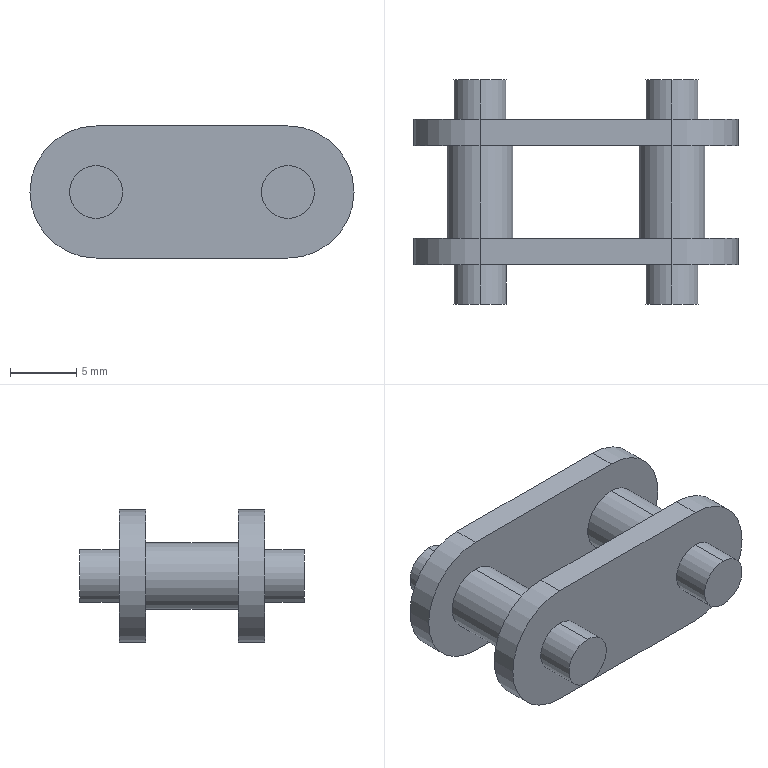Part | SolidWorks | features ICE 4, RefPoint 2, Extrusion 1 | 1 solid | 28 faces | box 24.52 x 17 x 10 mm | volume 1321 mm3 | cylinder 16 | plane 12 | commonest cylinder face diameters 4 x8 5 x4 10 x4
STEP:
#1=CARTESIAN_POINT('',(0.,-3.,-2.));
#2=VERTEX_POINT('',#1);
#3=CARTESIAN_POINT('',(0.,-3.,2.));
#4=VERTEX_POINT('',#3);
#5=CARTESIAN_POINT('',(0.,-3.,0.));
#6=DIRECTION('',(0.,-1.,0.));
#7=DIRECTION('',(0.,0.,-1.));
#8=AXIS2_PLACEMENT_3D('',#5,#6,#7);
#9=CIRCLE('',#8,2.);
#10=EDGE_CURVE('',#2,#4,#9,.T.);
#11=ORIENTED_EDGE('',*,*,#10,.F.);
#12=CARTESIAN_POINT('',(0.,0.,-2.));
#13=VERTEX_POINT('',#12);
#14=CARTESIAN_POINT('',(0.,-3.,-2.));
#15=DIRECTION('',(0.,1.,0.));
#16=VECTOR('',#15,1000.);
#17=LINE('',#14,#16);
#18=EDGE_CURVE('',#2,#13,#17,.T.);
#19=ORIENTED_EDGE('',*,*,#18,.T.);
#20=CARTESIAN_POINT('',(0.,0.,2.));
#21=VERTEX_POINT('',#20);
#22=CARTESIAN_POINT('',(0.,0.,0.));
#23=DIRECTION('',(0.,-1.,0.));
#24=DIRECTION('',(0.,0.,1.));
#25=AXIS2_PLACEMENT_3D('',#22,#23,#24);
#26=CIRCLE('',#25,2.);
#27=EDGE_CURVE('',#13,#21,#26,.T.);
#28=ORIENTED_EDGE('',*,*,#27,.T.);
#29=CARTESIAN_POINT('',(0.,-3.,2.));
#30=DIRECTION('',(0.,1.,0.));
#31=VECTOR('',#30,1000.);
#32=LINE('',#29,#31);
#33=EDGE_CURVE('',#4,#21,#32,.T.);
#34=ORIENTED_EDGE('',*,*,#33,.F.);
#35=EDGE_LOOP('',(#11,#19,#28,#34));
#36=FACE_OUTER_BOUND('',#35,.T.);
#37=CARTESIAN_POINT('',(0.,-3.,0.));
#38=DIRECTION('',(0.,1.,0.));
#39=DIRECTION('',(0.,0.,1.));
#40=AXIS2_PLACEMENT_3D('',#37,#38,#39);
#41=CYLINDRICAL_SURFACE('',#40,2.);
#42=ADVANCED_FACE('',(#36),#41,.T.);
#43=CARTESIAN_POINT('',(14.52,-3.,-2.));
#44=VERTEX_POINT('',#43);
#45=CARTESIAN_POINT('',(14.52,-3.,2.));
#46=VERTEX_POINT('',#45);
#47=CARTESIAN_POINT('',(14.52,-3.,0.));
#48=DIRECTION('',(0.,-1.,0.));
#49=DIRECTION('',(0.,0.,-1.));
#50=AXIS2_PLACEMENT_3D('',#47,#48,#49);
#51=CIRCLE('',#50,2.);
#52=EDGE_CURVE('',#44,#46,#51,.T.);
#53=ORIENTED_EDGE('',*,*,#52,.F.);
#54=CARTESIAN_POINT('',(14.52,0.,-2.));
#55=VERTEX_POINT('',#54);
#56=CARTESIAN_POINT('',(14.52,-3.,-2.));
#57=DIRECTION('',(0.,1.,0.));
#58=VECTOR('',#57,1000.);
#59=LINE('',#56,#58);
#60=EDGE_CURVE('',#44,#55,#59,.T.);
#61=ORIENTED_EDGE('',*,*,#60,.T.);
#62=CARTESIAN_POINT('',(14.52,0.,2.));
#63=VERTEX_POINT('',#62);
#64=CARTESIAN_POINT('',(14.52,0.,0.));
#65=DIRECTION('',(0.,-1.,0.));
#66=DIRECTION('',(0.,0.,1.));
#67=AXIS2_PLACEMENT_3D('',#64,#65,#66);
#68=CIRCLE('',#67,2.);
#69=EDGE_CURVE('',#55,#63,#68,.T.);
#70=ORIENTED_EDGE('',*,*,#69,.T.);
#71=CARTESIAN_POINT('',(14.52,-3.,2.));
#72=DIRECTION('',(0.,1.,0.));
#73=VECTOR('',#72,1000.);
#74=LINE('',#71,#73);
#75=EDGE_CURVE('',#46,#63,#74,.T.);
#76=ORIENTED_EDGE('',*,*,#75,.F.);
#77=EDGE_LOOP('',(#53,#61,#70,#76));
#78=FACE_OUTER_BOUND('',#77,.T.);
#79=CARTESIAN_POINT('',(14.52,-3.,0.));
#80=DIRECTION('',(0.,1.,0.));
#81=DIRECTION('',(0.,0.,1.));
#82=AXIS2_PLACEMENT_3D('',#79,#80,#81);
#83=CYLINDRICAL_SURFACE('',#82,2.);
#84=ADVANCED_FACE('',(#78),#83,.T.);
#85=CARTESIAN_POINT('',(0.,14.,2.));
#86=VERTEX_POINT('',#85);
#87=CARTESIAN_POINT('',(0.,14.,-2.));
#88=VERTEX_POINT('',#87);
#89=CARTESIAN_POINT('',(0.,14.,0.));
#90=DIRECTION('',(0.,1.,0.));
#91=DIRECTION('',(0.,0.,1.));
#92=AXIS2_PLACEMENT_3D('',#89,#90,#91);
#93=CIRCLE('',#92,2.);
#94=EDGE_CURVE('',#86,#88,#93,.T.);
#95=ORIENTED_EDGE('',*,*,#94,.F.);
#96=CARTESIAN_POINT('',(0.,11.,2.));
#97=VERTEX_POINT('',#96);
#98=CARTESIAN_POINT('',(0.,14.,2.));
#99=DIRECTION('',(0.,-1.,0.));
#100=VECTOR('',#99,1000.);
#101=LINE('',#98,#100);
#102=EDGE_CURVE('',#86,#97,#101,.T.);
#103=ORIENTED_EDGE('',*,*,#102,.T.);
#104=CARTESIAN_POINT('',(0.,11.,-2.));
#105=VERTEX_POINT('',#104);
#106=CARTESIAN_POINT('',(0.,11.,0.));
#107=DIRECTION('',(0.,1.,0.));
#108=DIRECTION('',(0.,0.,1.));
#109=AXIS2_PLACEMENT_3D('',#106,#107,#108);
#110=CIRCLE('',#109,2.);
#111=EDGE_CURVE('',#97,#105,#110,.T.);
#112=ORIENTED_EDGE('',*,*,#111,.T.);
#113=CARTESIAN_POINT('',(0.,14.,-2.));
#114=DIRECTION('',(0.,-1.,0.));
#115=VECTOR('',#114,1000.);
#116=LINE('',#113,#115);
#117=EDGE_CURVE('',#88,#105,#116,.T.);
#118=ORIENTED_EDGE('',*,*,#117,.F.);
#119=EDGE_LOOP('',(#95,#103,#112,#118));
#120=FACE_OUTER_BOUND('',#119,.T.);
#121=CARTESIAN_POINT('',(0.,14.,0.));
#122=DIRECTION('',(0.,-1.,0.));
#123=DIRECTION('',(0.,0.,-1.));
#124=AXIS2_PLACEMENT_3D('',#121,#122,#123);
#125=CYLINDRICAL_SURFACE('',#124,2.);
#126=ADVANCED_FACE('',(#120),#125,.T.);
#127=CARTESIAN_POINT('',(14.52,14.,2.));
#128=VERTEX_POINT('',#127);
#129=CARTESIAN_POINT('',(14.52,14.,-2.));
#130=VERTEX_POINT('',#129);
#131=CARTESIAN_POINT('',(14.52,14.,0.));
#132=DIRECTION('',(0.,1.,0.));
#133=DIRECTION('',(0.,0.,1.));
#134=AXIS2_PLACEMENT_3D('',#131,#132,#133);
#135=CIRCLE('',#134,2.);
#136=EDGE_CURVE('',#128,#130,#135,.T.);
#137=ORIENTED_EDGE('',*,*,#136,.F.);
#138=CARTESIAN_POINT('',(14.52,11.,2.));
#139=VERTEX_POINT('',#138);
#140=CARTESIAN_POINT('',(14.52,14.,2.));
#141=DIRECTION('',(0.,-1.,0.));
#142=VECTOR('',#141,1000.);
#143=LINE('',#140,#142);
#144=EDGE_CURVE('',#128,#139,#143,.T.);
#145=ORIENTED_EDGE('',*,*,#144,.T.);
#146=CARTESIAN_POINT('',(14.52,11.,-2.));
#147=VERTEX_POINT('',#146);
#148=CARTESIAN_POINT('',(14.52,11.,0.));
#149=DIRECTION('',(0.,1.,0.));
#150=DIRECTION('',(0.,0.,1.));
#151=AXIS2_PLACEMENT_3D('',#148,#149,#150);
#152=CIRCLE('',#151,2.);
#153=EDGE_CURVE('',#139,#147,#152,.T.);
#154=ORIENTED_EDGE('',*,*,#153,.T.);
#155=CARTESIAN_POINT('',(14.52,14.,-2.));
#156=DIRECTION('',(0.,-1.,0.));
#157=VECTOR('',#156,1000.);
#158=LINE('',#155,#157);
#159=EDGE_CURVE('',#130,#147,#158,.T.);
#160=ORIENTED_EDGE('',*,*,#159,.F.);
#161=EDGE_LOOP('',(#137,#145,#154,#160));
#162=FACE_OUTER_BOUND('',#161,.T.);
#163=CARTESIAN_POINT('',(14.52,14.,0.));
#164=DIRECTION('',(0.,-1.,0.));
#165=DIRECTION('',(0.,0.,-1.));
#166=AXIS2_PLACEMENT_3D('',#163,#164,#165);
#167=CYLINDRICAL_SURFACE('',#166,2.);
#168=ADVANCED_FACE('',(#162),#167,.T.);
#169=CARTESIAN_POINT('',(0.,9.,2.5));
#170=VERTEX_POINT('',#169);
#171=CARTESIAN_POINT('',(0.,9.,-2.5));
#172=VERTEX_POINT('',#171);
#173=CARTESIAN_POINT('',(0.,9.,0.));
#174=DIRECTION('',(0.,1.,0.));
#175=DIRECTION('',(0.,0.,1.));
#176=AXIS2_PLACEMENT_3D('',#173,#174,#175);
#177=CIRCLE('',#176,2.5);
#178=EDGE_CURVE('',#170,#172,#177,.T.);
#179=ORIENTED_EDGE('',*,*,#178,.F.);
#180=CARTESIAN_POINT('',(0.,2.,2.5));
#181=VERTEX_POINT('',#180);
#182=CARTESIAN_POINT('',(0.,9.,2.5));
#183=DIRECTION('',(0.,-1.,0.));
#184=VECTOR('',#183,1000.);
#185=LINE('',#182,#184);
#186=EDGE_CURVE('',#170,#181,#185,.T.);
#187=ORIENTED_EDGE('',*,*,#186,.T.);
#188=CARTESIAN_POINT('',(0.,2.,-2.5));
#189=VERTEX_POINT('',#188);
#190=CARTESIAN_POINT('',(0.,2.,0.));
#191=DIRECTION('',(0.,1.,0.));
#192=DIRECTION('',(0.,0.,1.));
#193=AXIS2_PLACEMENT_3D('',#190,#191,#192);
#194=CIRCLE('',#193,2.5);
#195=EDGE_CURVE('',#181,#189,#194,.T.);
#196=ORIENTED_EDGE('',*,*,#195,.T.);
#197=CARTESIAN_POINT('',(0.,9.,-2.5));
#198=DIRECTION('',(0.,-1.,0.));
#199=VECTOR('',#198,1000.);
#200=LINE('',#197,#199);
#201=EDGE_CURVE('',#172,#189,#200,.T.);
#202=ORIENTED_EDGE('',*,*,#201,.F.);
#203=EDGE_LOOP('',(#179,#187,#196,#202));
#204=FACE_OUTER_BOUND('',#203,.T.);
#205=CARTESIAN_POINT('',(0.,9.,0.));
#206=DIRECTION('',(0.,-1.,0.));
#207=DIRECTION('',(0.,0.,-1.));
#208=AXIS2_PLACEMENT_3D('',#205,#206,#207);
#209=CYLINDRICAL_SURFACE('',#208,2.5);
#210=ADVANCED_FACE('',(#204),#209,.T.);
#211=CARTESIAN_POINT('',(14.52,9.,2.5));
#212=VERTEX_POINT('',#211);
#213=CARTESIAN_POINT('',(14.52,9.,-2.5));
#214=VERTEX_POINT('',#213);
#215=CARTESIAN_POINT('',(14.52,9.,0.));
#216=DIRECTION('',(0.,1.,0.));
#217=DIRECTION('',(0.,0.,1.));
#218=AXIS2_PLACEMENT_3D('',#215,#216,#217);
#219=CIRCLE('',#218,2.5);
#220=EDGE_CURVE('',#212,#214,#219,.T.);
#221=ORIENTED_EDGE('',*,*,#220,.F.);
#222=CARTESIAN_POINT('',(14.52,2.,2.5));
#223=VERTEX_POINT('',#222);
#224=CARTESIAN_POINT('',(14.52,9.,2.5));
#225=DIRECTION('',(0.,-1.,0.));
#226=VECTOR('',#225,1000.);
#227=LINE('',#224,#226);
#228=EDGE_CURVE('',#212,#223,#227,.T.);
#229=ORIENTED_EDGE('',*,*,#228,.T.);
#230=CARTESIAN_POINT('',(14.52,2.,-2.5));
#231=VERTEX_POINT('',#230);
#232=CARTESIAN_POINT('',(14.52,2.,0.));
#233=DIRECTION('',(0.,1.,0.));
#234=DIRECTION('',(0.,0.,1.));
#235=AXIS2_PLACEMENT_3D('',#232,#233,#234);
#236=CIRCLE('',#235,2.5);
#237=EDGE_CURVE('',#223,#231,#236,.T.);
#238=ORIENTED_EDGE('',*,*,#237,.T.);
#239=CARTESIAN_POINT('',(14.52,9.,-2.5));
#240=DIRECTION('',(0.,-1.,0.));
#241=VECTOR('',#240,1000.);
#242=LINE('',#239,#241);
#243=EDGE_CURVE('',#214,#231,#242,.T.);
#244=ORIENTED_EDGE('',*,*,#243,.F.);
#245=EDGE_LOOP('',(#221,#229,#238,#244));
#246=FACE_OUTER_BOUND('',#245,.T.);
#247=CARTESIAN_POINT('',(14.52,9.,0.));
#248=DIRECTION('',(0.,-1.,0.));
#249=DIRECTION('',(0.,0.,-1.));
#250=AXIS2_PLACEMENT_3D('',#247,#248,#249);
#251=CYLINDRICAL_SURFACE('',#250,2.5);
#252=ADVANCED_FACE('',(#246),#251,.T.);
#253=CARTESIAN_POINT('',(0.,0.,-5.));
#254=VERTEX_POINT('',#253);
#255=CARTESIAN_POINT('',(0.,0.,5.));
#256=VERTEX_POINT('',#255);
#257=CARTESIAN_POINT('',(0.,0.,0.));
#258=DIRECTION('',(0.,1.,0.));
#259=DIRECTION('',(0.,0.,1.));
#260=AXIS2_PLACEMENT_3D('',#257,#258,#259);
#261=CIRCLE('',#260,5.);
#262=EDGE_CURVE('',#254,#256,#261,.T.);
#263=ORIENTED_EDGE('',*,*,#262,.T.);
#264=CARTESIAN_POINT('',(0.,2.,5.));
#265=VERTEX_POINT('',#264);
#266=CARTESIAN_POINT('',(0.,2.,5.));
#267=DIRECTION('',(0.,-1.,0.));
#268=VECTOR('',#267,1000.);
#269=LINE('',#266,#268);
#270=EDGE_CURVE('',#265,#256,#269,.T.);
#271=ORIENTED_EDGE('',*,*,#270,.F.);
#272=CARTESIAN_POINT('',(0.,2.,-5.));
#273=VERTEX_POINT('',#272);
#274=CARTESIAN_POINT('',(0.,2.,0.));
#275=DIRECTION('',(0.,1.,0.));
#276=DIRECTION('',(0.,0.,1.));
#277=AXIS2_PLACEMENT_3D('',#274,#275,#276);
#278=CIRCLE('',#277,5.);
#279=EDGE_CURVE('',#273,#265,#278,.T.);
#280=ORIENTED_EDGE('',*,*,#279,.F.);
#281=CARTESIAN_POINT('',(0.,2.,-5.));
#282=DIRECTION('',(0.,-1.,0.));
#283=VECTOR('',#282,1000.);
#284=LINE('',#281,#283);
#285=EDGE_CURVE('',#273,#254,#284,.T.);
#286=ORIENTED_EDGE('',*,*,#285,.T.);
#287=EDGE_LOOP('',(#263,#271,#280,#286));
#288=FACE_OUTER_BOUND('',#287,.T.);
#289=CARTESIAN_POINT('',(0.,2.,0.));
#290=DIRECTION('',(0.,-1.,0.));
#291=DIRECTION('',(0.,0.,-1.));
#292=AXIS2_PLACEMENT_3D('',#289,#290,#291);
#293=CYLINDRICAL_SURFACE('',#292,5.);
#294=ADVANCED_FACE('',(#288),#293,.T.);
#295=CARTESIAN_POINT('',(14.52,0.,5.));
#296=VERTEX_POINT('',#295);
#297=CARTESIAN_POINT('',(0.,0.,5.));
#298=DIRECTION('',(1.,0.,0.));
#299=VECTOR('',#298,1000.);
#300=LINE('',#297,#299);
#301=EDGE_CURVE('',#256,#296,#300,.T.);
#302=ORIENTED_EDGE('',*,*,#301,.T.);
#303=CARTESIAN_POINT('',(14.52,2.,5.));
#304=VERTEX_POINT('',#303);
#305=CARTESIAN_POINT('',(14.52,2.,5.));
#306=DIRECTION('',(0.,-1.,0.));
#307=VECTOR('',#306,1000.);
#308=LINE('',#305,#307);
#309=EDGE_CURVE('',#304,#296,#308,.T.);
#310=ORIENTED_EDGE('',*,*,#309,.F.);
#311=CARTESIAN_POINT('',(0.,2.,5.));
#312=DIRECTION('',(1.,0.,0.));
#313=VECTOR('',#312,1000.);
#314=LINE('',#311,#313);
#315=EDGE_CURVE('',#265,#304,#314,.T.);
#316=ORIENTED_EDGE('',*,*,#315,.F.);
#317=ORIENTED_EDGE('',*,*,#270,.T.);
#318=EDGE_LOOP('',(#302,#310,#316,#317));
#319=FACE_OUTER_BOUND('',#318,.T.);
#320=CARTESIAN_POINT('',(0.,2.,5.));
#321=DIRECTION('',(0.,0.,-1.));
#322=DIRECTION('',(-1.,0.,0.));
#323=AXIS2_PLACEMENT_3D('',#320,#321,#322);
#324=PLANE('',#323);
#325=ADVANCED_FACE('',(#319),#324,.F.);
#326=CARTESIAN_POINT('',(14.52,0.,-5.));
#327=VERTEX_POINT('',#326);
#328=CARTESIAN_POINT('',(14.52,0.,0.));
#329=DIRECTION('',(0.,1.,0.));
#330=DIRECTION('',(0.,0.,1.));
#331=AXIS2_PLACEMENT_3D('',#328,#329,#330);
#332=CIRCLE('',#331,5.);
#333=EDGE_CURVE('',#296,#327,#332,.T.);
#334=ORIENTED_EDGE('',*,*,#333,.T.);
#335=CARTESIAN_POINT('',(14.52,2.,-5.));
#336=VERTEX_POINT('',#335);
#337=CARTESIAN_POINT('',(14.52,2.,-5.));
#338=DIRECTION('',(0.,-1.,0.));
#339=VECTOR('',#338,1000.);
#340=LINE('',#337,#339);
#341=EDGE_CURVE('',#336,#327,#340,.T.);
#342=ORIENTED_EDGE('',*,*,#341,.F.);
#343=CARTESIAN_POINT('',(14.52,2.,0.));
#344=DIRECTION('',(0.,1.,0.));
#345=DIRECTION('',(0.,0.,1.));
#346=AXIS2_PLACEMENT_3D('',#343,#344,#345);
#347=CIRCLE('',#346,5.);
#348=EDGE_CURVE('',#304,#336,#347,.T.);
#349=ORIENTED_EDGE('',*,*,#348,.F.);
#350=ORIENTED_EDGE('',*,*,#309,.T.);
#351=EDGE_LOOP('',(#334,#342,#349,#350));
#352=FACE_OUTER_BOUND('',#351,.T.);
#353=CARTESIAN_POINT('',(14.52,2.,0.));
#354=DIRECTION('',(0.,-1.,0.));
#355=DIRECTION('',(0.,0.,-1.));
#356=AXIS2_PLACEMENT_3D('',#353,#354,#355);
#357=CYLINDRICAL_SURFACE('',#356,5.);
#358=ADVANCED_FACE('',(#352),#357,.T.);
#359=CARTESIAN_POINT('',(0.,0.,-5.));
#360=DIRECTION('',(-1.,0.,0.));
#361=VECTOR('',#360,1000.);
#362=LINE('',#359,#361);
#363=EDGE_CURVE('',#327,#254,#362,.T.);
#364=ORIENTED_EDGE('',*,*,#363,.T.);
#365=ORIENTED_EDGE('',*,*,#285,.F.);
#366=CARTESIAN_POINT('',(0.,2.,-5.));
#367=DIRECTION('',(-1.,0.,0.));
#368=VECTOR('',#367,1000.);
#369=LINE('',#366,#368);
#370=EDGE_CURVE('',#336,#273,#369,.T.);
#371=ORIENTED_EDGE('',*,*,#370,.F.);
#372=ORIENTED_EDGE('',*,*,#341,.T.);
#373=EDGE_LOOP('',(#364,#365,#371,#372));
#374=FACE_OUTER_BOUND('',#373,.T.);
#375=CARTESIAN_POINT('',(0.,2.,-5.));
#376=DIRECTION('',(0.,0.,1.));
#377=DIRECTION('',(1.,0.,0.));
#378=AXIS2_PLACEMENT_3D('',#375,#376,#377);
#379=PLANE('',#378);
#380=ADVANCED_FACE('',(#374),#379,.F.);
#381=CARTESIAN_POINT('',(0.,2.,0.));
#382=DIRECTION('',(0.,1.,0.));
#383=DIRECTION('',(0.,0.,1.));
#384=AXIS2_PLACEMENT_3D('',#381,#382,#383);
#385=CIRCLE('',#384,2.5);
#386=EDGE_CURVE('',#189,#181,#385,.T.);
#387=ORIENTED_EDGE('',*,*,#386,.F.);
#388=ORIENTED_EDGE('',*,*,#195,.F.);
#389=EDGE_LOOP('',(#387,#388));
#390=FACE_BOUND('',#389,.T.);
#391=CARTESIAN_POINT('',(14.52,2.,0.));
#392=DIRECTION('',(0.,1.,0.));
#393=DIRECTION('',(0.,0.,1.));
#394=AXIS2_PLACEMENT_3D('',#391,#392,#393);
#395=CIRCLE('',#394,2.5);
#396=EDGE_CURVE('',#231,#223,#395,.T.);
#397=ORIENTED_EDGE('',*,*,#396,.F.);
#398=ORIENTED_EDGE('',*,*,#237,.F.);
#399=EDGE_LOOP('',(#397,#398));
#400=FACE_BOUND('',#399,.T.);
#401=ORIENTED_EDGE('',*,*,#279,.T.);
#402=ORIENTED_EDGE('',*,*,#315,.T.);
#403=ORIENTED_EDGE('',*,*,#348,.T.);
#404=ORIENTED_EDGE('',*,*,#370,.T.);
#405=EDGE_LOOP('',(#401,#402,#403,#404));
#406=FACE_OUTER_BOUND('',#405,.T.);
#407=CARTESIAN_POINT('',(0.,2.,0.));
#408=DIRECTION('',(0.,1.,0.));
#409=DIRECTION('',(0.,0.,1.));
#410=AXIS2_PLACEMENT_3D('',#407,#408,#409);
#411=PLANE('',#410);
#412=ADVANCED_FACE('',(#390,#400,#406),#411,.T.);
#413=CARTESIAN_POINT('',(0.,0.,0.));
#414=DIRECTION('',(0.,-1.,0.));
#415=DIRECTION('',(0.,0.,1.));
#416=AXIS2_PLACEMENT_3D('',#413,#414,#415);
#417=CIRCLE('',#416,2.);
#418=EDGE_CURVE('',#21,#13,#417,.T.);
#419=ORIENTED_EDGE('',*,*,#418,.F.);
#420=ORIENTED_EDGE('',*,*,#27,.F.);
#421=EDGE_LOOP('',(#419,#420));
#422=FACE_BOUND('',#421,.T.);
#423=CARTESIAN_POINT('',(14.52,0.,0.));
#424=DIRECTION('',(0.,-1.,0.));
#425=DIRECTION('',(0.,0.,1.));
#426=AXIS2_PLACEMENT_3D('',#423,#424,#425);
#427=CIRCLE('',#426,2.);
#428=EDGE_CURVE('',#63,#55,#427,.T.);
#429=ORIENTED_EDGE('',*,*,#428,.F.);
#430=ORIENTED_EDGE('',*,*,#69,.F.);
#431=EDGE_LOOP('',(#429,#430));
#432=FACE_BOUND('',#431,.T.);
#433=ORIENTED_EDGE('',*,*,#262,.F.);
#434=ORIENTED_EDGE('',*,*,#363,.F.);
#435=ORIENTED_EDGE('',*,*,#333,.F.);
#436=ORIENTED_EDGE('',*,*,#301,.F.);
#437=EDGE_LOOP('',(#433,#434,#435,#436));
#438=FACE_OUTER_BOUND('',#437,.T.);
#439=CARTESIAN_POINT('',(0.,0.,0.));
#440=DIRECTION('',(0.,1.,0.));
#441=DIRECTION('',(0.,0.,1.));
#442=AXIS2_PLACEMENT_3D('',#439,#440,#441);
#443=PLANE('',#442);
#444=ADVANCED_FACE('',(#422,#432,#438),#443,.F.);
#445=ORIENTED_EDGE('',*,*,#228,.F.);
#446=CARTESIAN_POINT('',(14.52,9.,0.));
#447=DIRECTION('',(0.,1.,0.));
#448=DIRECTION('',(0.,0.,1.));
#449=AXIS2_PLACEMENT_3D('',#446,#447,#448);
#450=CIRCLE('',#449,2.5);
#451=EDGE_CURVE('',#214,#212,#450,.T.);
#452=ORIENTED_EDGE('',*,*,#451,.F.);
#453=ORIENTED_EDGE('',*,*,#243,.T.);
#454=ORIENTED_EDGE('',*,*,#396,.T.);
#455=EDGE_LOOP('',(#445,#452,#453,#454));
#456=FACE_OUTER_BOUND('',#455,.T.);
#457=CARTESIAN_POINT('',(14.52,9.,0.));
#458=DIRECTION('',(0.,-1.,0.));
#459=DIRECTION('',(0.,0.,-1.));
#460=AXIS2_PLACEMENT_3D('',#457,#458,#459);
#461=CYLINDRICAL_SURFACE('',#460,2.5);
#462=ADVANCED_FACE('',(#456),#461,.T.);
#463=ORIENTED_EDGE('',*,*,#186,.F.);
#464=CARTESIAN_POINT('',(0.,9.,0.));
#465=DIRECTION('',(0.,1.,0.));
#466=DIRECTION('',(0.,0.,1.));
#467=AXIS2_PLACEMENT_3D('',#464,#465,#466);
#468=CIRCLE('',#467,2.5);
#469=EDGE_CURVE('',#172,#170,#468,.T.);
#470=ORIENTED_EDGE('',*,*,#469,.F.);
#471=ORIENTED_EDGE('',*,*,#201,.T.);
#472=ORIENTED_EDGE('',*,*,#386,.T.);
#473=EDGE_LOOP('',(#463,#470,#471,#472));
#474=FACE_OUTER_BOUND('',#473,.T.);
#475=CARTESIAN_POINT('',(0.,9.,0.));
#476=DIRECTION('',(0.,-1.,0.));
#477=DIRECTION('',(0.,0.,-1.));
#478=AXIS2_PLACEMENT_3D('',#475,#476,#477);
#479=CYLINDRICAL_SURFACE('',#478,2.5);
#480=ADVANCED_FACE('',(#474),#479,.T.);
#481=CARTESIAN_POINT('',(0.,9.,-5.));
#482=VERTEX_POINT('',#481);
#483=CARTESIAN_POINT('',(0.,9.,5.));
#484=VERTEX_POINT('',#483);
#485=CARTESIAN_POINT('',(0.,9.,0.));
#486=DIRECTION('',(0.,1.,0.));
#487=DIRECTION('',(0.,0.,1.));
#488=AXIS2_PLACEMENT_3D('',#485,#486,#487);
#489=CIRCLE('',#488,5.);
#490=EDGE_CURVE('',#482,#484,#489,.T.);
#491=ORIENTED_EDGE('',*,*,#490,.T.);
#492=CARTESIAN_POINT('',(0.,11.,5.));
#493=VERTEX_POINT('',#492);
#494=CARTESIAN_POINT('',(0.,11.,5.));
#495=DIRECTION('',(0.,-1.,0.));
#496=VECTOR('',#495,1000.);
#497=LINE('',#494,#496);
#498=EDGE_CURVE('',#493,#484,#497,.T.);
#499=ORIENTED_EDGE('',*,*,#498,.F.);
#500=CARTESIAN_POINT('',(0.,11.,-5.));
#501=VERTEX_POINT('',#500);
#502=CARTESIAN_POINT('',(0.,11.,0.));
#503=DIRECTION('',(0.,1.,0.));
#504=DIRECTION('',(0.,0.,1.));
#505=AXIS2_PLACEMENT_3D('',#502,#503,#504);
#506=CIRCLE('',#505,5.);
#507=EDGE_CURVE('',#501,#493,#506,.T.);
#508=ORIENTED_EDGE('',*,*,#507,.F.);
#509=CARTESIAN_POINT('',(0.,11.,-5.));
#510=DIRECTION('',(0.,-1.,0.));
#511=VECTOR('',#510,1000.);
#512=LINE('',#509,#511);
#513=EDGE_CURVE('',#501,#482,#512,.T.);
#514=ORIENTED_EDGE('',*,*,#513,.T.);
#515=EDGE_LOOP('',(#491,#499,#508,#514));
#516=FACE_OUTER_BOUND('',#515,.T.);
#517=CARTESIAN_POINT('',(0.,11.,0.));
#518=DIRECTION('',(0.,-1.,0.));
#519=DIRECTION('',(0.,0.,-1.));
#520=AXIS2_PLACEMENT_3D('',#517,#518,#519);
#521=CYLINDRICAL_SURFACE('',#520,5.);
#522=ADVANCED_FACE('',(#516),#521,.T.);
#523=CARTESIAN_POINT('',(14.52,9.,5.));
#524=VERTEX_POINT('',#523);
#525=CARTESIAN_POINT('',(0.,9.,5.));
#526=DIRECTION('',(1.,0.,0.));
#527=VECTOR('',#526,1000.);
#528=LINE('',#525,#527);
#529=EDGE_CURVE('',#484,#524,#528,.T.);
#530=ORIENTED_EDGE('',*,*,#529,.T.);
#531=CARTESIAN_POINT('',(14.52,11.,5.));
#532=VERTEX_POINT('',#531);
#533=CARTESIAN_POINT('',(14.52,11.,5.));
#534=DIRECTION('',(0.,-1.,0.));
#535=VECTOR('',#534,1000.);
#536=LINE('',#533,#535);
#537=EDGE_CURVE('',#532,#524,#536,.T.);
#538=ORIENTED_EDGE('',*,*,#537,.F.);
#539=CARTESIAN_POINT('',(0.,11.,5.));
#540=DIRECTION('',(1.,0.,0.));
#541=VECTOR('',#540,1000.);
#542=LINE('',#539,#541);
#543=EDGE_CURVE('',#493,#532,#542,.T.);
#544=ORIENTED_EDGE('',*,*,#543,.F.);
#545=ORIENTED_EDGE('',*,*,#498,.T.);
#546=EDGE_LOOP('',(#530,#538,#544,#545));
#547=FACE_OUTER_BOUND('',#546,.T.);
#548=CARTESIAN_POINT('',(0.,11.,5.));
#549=DIRECTION('',(0.,0.,-1.));
#550=DIRECTION('',(-1.,0.,0.));
#551=AXIS2_PLACEMENT_3D('',#548,#549,#550);
#552=PLANE('',#551);
#553=ADVANCED_FACE('',(#547),#552,.F.);
#554=CARTESIAN_POINT('',(14.52,9.,-5.));
#555=VERTEX_POINT('',#554);
#556=CARTESIAN_POINT('',(14.52,9.,0.));
#557=DIRECTION('',(0.,1.,0.));
#558=DIRECTION('',(0.,0.,1.));
#559=AXIS2_PLACEMENT_3D('',#556,#557,#558);
#560=CIRCLE('',#559,5.);
#561=EDGE_CURVE('',#524,#555,#560,.T.);
#562=ORIENTED_EDGE('',*,*,#561,.T.);
#563=CARTESIAN_POINT('',(14.52,11.,-5.));
#564=VERTEX_POINT('',#563);
#565=CARTESIAN_POINT('',(14.52,11.,-5.));
#566=DIRECTION('',(0.,-1.,0.));
#567=VECTOR('',#566,1000.);
#568=LINE('',#565,#567);
#569=EDGE_CURVE('',#564,#555,#568,.T.);
#570=ORIENTED_EDGE('',*,*,#569,.F.);
#571=CARTESIAN_POINT('',(14.52,11.,0.));
#572=DIRECTION('',(0.,1.,0.));
#573=DIRECTION('',(0.,0.,1.));
#574=AXIS2_PLACEMENT_3D('',#571,#572,#573);
#575=CIRCLE('',#574,5.);
#576=EDGE_CURVE('',#532,#564,#575,.T.);
#577=ORIENTED_EDGE('',*,*,#576,.F.);
#578=ORIENTED_EDGE('',*,*,#537,.T.);
#579=EDGE_LOOP('',(#562,#570,#577,#578));
#580=FACE_OUTER_BOUND('',#579,.T.);
#581=CARTESIAN_POINT('',(14.52,11.,0.));
#582=DIRECTION('',(0.,-1.,0.));
#583=DIRECTION('',(0.,0.,-1.));
#584=AXIS2_PLACEMENT_3D('',#581,#582,#583);
#585=CYLINDRICAL_SURFACE('',#584,5.);
#586=ADVANCED_FACE('',(#580),#585,.T.);
#587=CARTESIAN_POINT('',(0.,9.,-5.));
#588=DIRECTION('',(-1.,0.,0.));
#589=VECTOR('',#588,1000.);
#590=LINE('',#587,#589);
#591=EDGE_CURVE('',#555,#482,#590,.T.);
#592=ORIENTED_EDGE('',*,*,#591,.T.);
#593=ORIENTED_EDGE('',*,*,#513,.F.);
#594=CARTESIAN_POINT('',(0.,11.,-5.));
#595=DIRECTION('',(-1.,0.,0.));
#596=VECTOR('',#595,1000.);
#597=LINE('',#594,#596);
#598=EDGE_CURVE('',#564,#501,#597,.T.);
#599=ORIENTED_EDGE('',*,*,#598,.F.);
#600=ORIENTED_EDGE('',*,*,#569,.T.);
#601=EDGE_LOOP('',(#592,#593,#599,#600));
#602=FACE_OUTER_BOUND('',#601,.T.);
#603=CARTESIAN_POINT('',(0.,11.,-5.));
#604=DIRECTION('',(0.,0.,1.));
#605=DIRECTION('',(1.,0.,0.));
#606=AXIS2_PLACEMENT_3D('',#603,#604,#605);
#607=PLANE('',#606);
#608=ADVANCED_FACE('',(#602),#607,.F.);
#609=CARTESIAN_POINT('',(0.,11.,0.));
#610=DIRECTION('',(0.,1.,0.));
#611=DIRECTION('',(0.,0.,1.));
#612=AXIS2_PLACEMENT_3D('',#609,#610,#611);
#613=CIRCLE('',#612,2.);
#614=EDGE_CURVE('',#105,#97,#613,.T.);
#615=ORIENTED_EDGE('',*,*,#614,.F.);
#616=ORIENTED_EDGE('',*,*,#111,.F.);
#617=EDGE_LOOP('',(#615,#616));
#618=FACE_BOUND('',#617,.T.);
#619=CARTESIAN_POINT('',(14.52,11.,0.));
#620=DIRECTION('',(0.,1.,0.));
#621=DIRECTION('',(0.,0.,1.));
#622=AXIS2_PLACEMENT_3D('',#619,#620,#621);
#623=CIRCLE('',#622,2.);
#624=EDGE_CURVE('',#147,#139,#623,.T.);
#625=ORIENTED_EDGE('',*,*,#624,.F.);
#626=ORIENTED_EDGE('',*,*,#153,.F.);
#627=EDGE_LOOP('',(#625,#626));
#628=FACE_BOUND('',#627,.T.);
#629=ORIENTED_EDGE('',*,*,#507,.T.);
#630=ORIENTED_EDGE('',*,*,#543,.T.);
#631=ORIENTED_EDGE('',*,*,#576,.T.);
#632=ORIENTED_EDGE('',*,*,#598,.T.);
#633=EDGE_LOOP('',(#629,#630,#631,#632));
#634=FACE_OUTER_BOUND('',#633,.T.);
#635=CARTESIAN_POINT('',(0.,11.,0.));
#636=DIRECTION('',(0.,1.,0.));
#637=DIRECTION('',(0.,0.,1.));
#638=AXIS2_PLACEMENT_3D('',#635,#636,#637);
#639=PLANE('',#638);
#640=ADVANCED_FACE('',(#618,#628,#634),#639,.T.);
#641=ORIENTED_EDGE('',*,*,#451,.T.);
#642=ORIENTED_EDGE('',*,*,#220,.T.);
#643=EDGE_LOOP('',(#641,#642));
#644=FACE_BOUND('',#643,.T.);
#645=ORIENTED_EDGE('',*,*,#469,.T.);
#646=ORIENTED_EDGE('',*,*,#178,.T.);
#647=EDGE_LOOP('',(#645,#646));
#648=FACE_BOUND('',#647,.T.);
#649=ORIENTED_EDGE('',*,*,#490,.F.);
#650=ORIENTED_EDGE('',*,*,#591,.F.);
#651=ORIENTED_EDGE('',*,*,#561,.F.);
#652=ORIENTED_EDGE('',*,*,#529,.F.);
#653=EDGE_LOOP('',(#649,#650,#651,#652));
#654=FACE_OUTER_BOUND('',#653,.T.);
#655=CARTESIAN_POINT('',(0.,9.,0.));
#656=DIRECTION('',(0.,1.,0.));
#657=DIRECTION('',(0.,0.,1.));
#658=AXIS2_PLACEMENT_3D('',#655,#656,#657);
#659=PLANE('',#658);
#660=ADVANCED_FACE('',(#644,#648,#654),#659,.F.);
#661=ORIENTED_EDGE('',*,*,#144,.F.);
#662=CARTESIAN_POINT('',(14.52,14.,0.));
#663=DIRECTION('',(0.,1.,0.));
#664=DIRECTION('',(0.,0.,1.));
#665=AXIS2_PLACEMENT_3D('',#662,#663,#664);
#666=CIRCLE('',#665,2.);
#667=EDGE_CURVE('',#130,#128,#666,.T.);
#668=ORIENTED_EDGE('',*,*,#667,.F.);
#669=ORIENTED_EDGE('',*,*,#159,.T.);
#670=ORIENTED_EDGE('',*,*,#624,.T.);
#671=EDGE_LOOP('',(#661,#668,#669,#670));
#672=FACE_OUTER_BOUND('',#671,.T.);
#673=CARTESIAN_POINT('',(14.52,14.,0.));
#674=DIRECTION('',(0.,-1.,0.));
#675=DIRECTION('',(0.,0.,-1.));
#676=AXIS2_PLACEMENT_3D('',#673,#674,#675);
#677=CYLINDRICAL_SURFACE('',#676,2.);
#678=ADVANCED_FACE('',(#672),#677,.T.);
#679=ORIENTED_EDGE('',*,*,#667,.T.);
#680=ORIENTED_EDGE('',*,*,#136,.T.);
#681=EDGE_LOOP('',(#679,#680));
#682=FACE_OUTER_BOUND('',#681,.T.);
#683=CARTESIAN_POINT('',(14.52,14.,0.));
#684=DIRECTION('',(0.,1.,0.));
#685=DIRECTION('',(0.,0.,1.));
#686=AXIS2_PLACEMENT_3D('',#683,#684,#685);
#687=PLANE('',#686);
#688=ADVANCED_FACE('',(#682),#687,.T.);
#689=ORIENTED_EDGE('',*,*,#102,.F.);
#690=CARTESIAN_POINT('',(0.,14.,0.));
#691=DIRECTION('',(0.,1.,0.));
#692=DIRECTION('',(0.,0.,1.));
#693=AXIS2_PLACEMENT_3D('',#690,#691,#692);
#694=CIRCLE('',#693,2.);
#695=EDGE_CURVE('',#88,#86,#694,.T.);
#696=ORIENTED_EDGE('',*,*,#695,.F.);
#697=ORIENTED_EDGE('',*,*,#117,.T.);
#698=ORIENTED_EDGE('',*,*,#614,.T.);
#699=EDGE_LOOP('',(#689,#696,#697,#698));
#700=FACE_OUTER_BOUND('',#699,.T.);
#701=CARTESIAN_POINT('',(0.,14.,0.));
#702=DIRECTION('',(0.,-1.,0.));
#703=DIRECTION('',(0.,0.,-1.));
#704=AXIS2_PLACEMENT_3D('',#701,#702,#703);
#705=CYLINDRICAL_SURFACE('',#704,2.);
#706=ADVANCED_FACE('',(#700),#705,.T.);
#707=ORIENTED_EDGE('',*,*,#695,.T.);
#708=ORIENTED_EDGE('',*,*,#94,.T.);
#709=EDGE_LOOP('',(#707,#708));
#710=FACE_OUTER_BOUND('',#709,.T.);
#711=CARTESIAN_POINT('',(0.,14.,0.));
#712=DIRECTION('',(0.,1.,0.));
#713=DIRECTION('',(0.,0.,1.));
#714=AXIS2_PLACEMENT_3D('',#711,#712,#713);
#715=PLANE('',#714);
#716=ADVANCED_FACE('',(#710),#715,.T.);
#717=ORIENTED_EDGE('',*,*,#60,.F.);
#718=CARTESIAN_POINT('',(14.52,-3.,0.));
#719=DIRECTION('',(0.,-1.,0.));
#720=DIRECTION('',(0.,0.,-1.));
#721=AXIS2_PLACEMENT_3D('',#718,#719,#720);
#722=CIRCLE('',#721,2.);
#723=EDGE_CURVE('',#46,#44,#722,.T.);
#724=ORIENTED_EDGE('',*,*,#723,.F.);
#725=ORIENTED_EDGE('',*,*,#75,.T.);
#726=ORIENTED_EDGE('',*,*,#428,.T.);
#727=EDGE_LOOP('',(#717,#724,#725,#726));
#728=FACE_OUTER_BOUND('',#727,.T.);
#729=CARTESIAN_POINT('',(14.52,-3.,0.));
#730=DIRECTION('',(0.,1.,0.));
#731=DIRECTION('',(0.,0.,1.));
#732=AXIS2_PLACEMENT_3D('',#729,#730,#731);
#733=CYLINDRICAL_SURFACE('',#732,2.);
#734=ADVANCED_FACE('',(#728),#733,.T.);
#735=ORIENTED_EDGE('',*,*,#723,.T.);
#736=ORIENTED_EDGE('',*,*,#52,.T.);
#737=EDGE_LOOP('',(#735,#736));
#738=FACE_OUTER_BOUND('',#737,.T.);
#739=CARTESIAN_POINT('',(14.52,-3.,0.));
#740=DIRECTION('',(0.,-1.,0.));
#741=DIRECTION('',(0.,0.,-1.));
#742=AXIS2_PLACEMENT_3D('',#739,#740,#741);
#743=PLANE('',#742);
#744=ADVANCED_FACE('',(#738),#743,.T.);
#745=ORIENTED_EDGE('',*,*,#18,.F.);
#746=CARTESIAN_POINT('',(0.,-3.,0.));
#747=DIRECTION('',(0.,-1.,0.));
#748=DIRECTION('',(0.,0.,-1.));
#749=AXIS2_PLACEMENT_3D('',#746,#747,#748);
#750=CIRCLE('',#749,2.);
#751=EDGE_CURVE('',#4,#2,#750,.T.);
#752=ORIENTED_EDGE('',*,*,#751,.F.);
#753=ORIENTED_EDGE('',*,*,#33,.T.);
#754=ORIENTED_EDGE('',*,*,#418,.T.);
#755=EDGE_LOOP('',(#745,#752,#753,#754));
#756=FACE_OUTER_BOUND('',#755,.T.);
#757=CARTESIAN_POINT('',(0.,-3.,0.));
#758=DIRECTION('',(0.,1.,0.));
#759=DIRECTION('',(0.,0.,1.));
#760=AXIS2_PLACEMENT_3D('',#757,#758,#759);
#761=CYLINDRICAL_SURFACE('',#760,2.);
#762=ADVANCED_FACE('',(#756),#761,.T.);
#763=ORIENTED_EDGE('',*,*,#751,.T.);
#764=ORIENTED_EDGE('',*,*,#10,.T.);
#765=EDGE_LOOP('',(#763,#764));
#766=FACE_OUTER_BOUND('',#765,.T.);
#767=CARTESIAN_POINT('',(0.,-3.,0.));
#768=DIRECTION('',(0.,-1.,0.));
#769=DIRECTION('',(0.,0.,-1.));
#770=AXIS2_PLACEMENT_3D('',#767,#768,#769);
#771=PLANE('',#770);
#772=ADVANCED_FACE('',(#766),#771,.T.);
#773=CLOSED_SHELL('',(#42,#84,#126,#168,#210,#252,#294,#325,#358,#380,#412,#444,#462,#480,#522,#553,#586,#608,#640,#660,#678,#688,#706,#716,#734,#744,#762,#772));
#774=MANIFOLD_SOLID_BREP('',#773);
#775=CARTESIAN_POINT('',(0.,0.,0.));
#776=DIRECTION('',(0.,0.,1.));
#777=DIRECTION('',(1.,0.,0.));
#778=AXIS2_PLACEMENT_3D('',#775,#776,#777);
#779=(LENGTH_UNIT()NAMED_UNIT(*)SI_UNIT(.MILLI.,.METRE.));
#780=UNCERTAINTY_MEASURE_WITH_UNIT(LENGTH_MEASURE(0.00001),#779,'','');
#781=(NAMED_UNIT(*)PLANE_ANGLE_UNIT()SI_UNIT($,.RADIAN.));
#782=(NAMED_UNIT(*)SI_UNIT($,.STERADIAN.)SOLID_ANGLE_UNIT());
#783=(GEOMETRIC_REPRESENTATION_CONTEXT(3)GLOBAL_UNCERTAINTY_ASSIGNED_CONTEXT((#780))GLOBAL_UNIT_ASSIGNED_CONTEXT((#779,#781,#782))REPRESENTATION_CONTEXT('',''));
#784=ADVANCED_BREP_SHAPE_REPRESENTATION('',(#774,#778),#783);